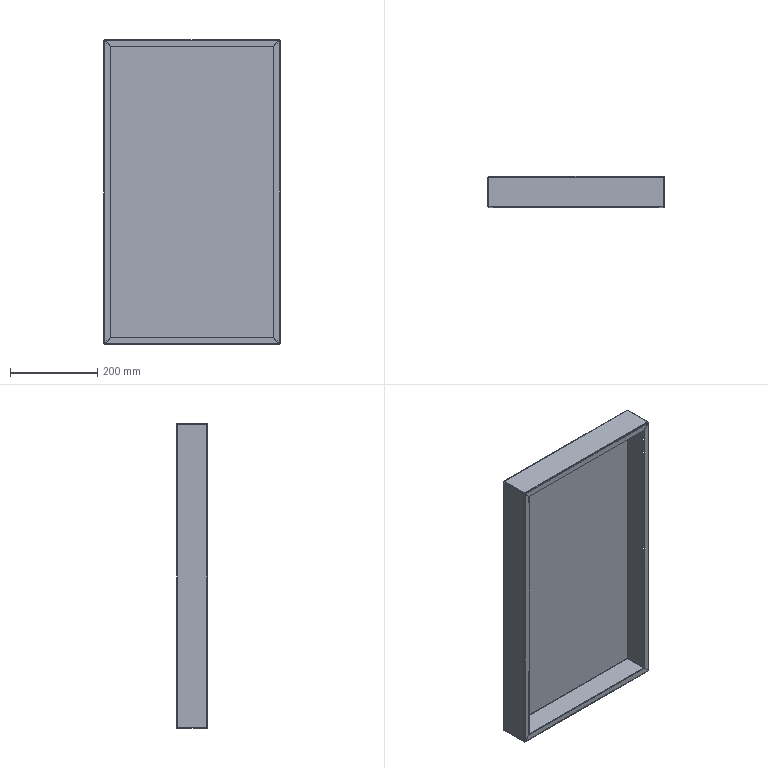Part | SolidWorks | features BaseBody 1 | 1 solid | 78 faces | box 405 x 70 x 700 mm | volume 689241 mm3 | plane 38 | cylinder 24 | spline 16 | commonest cylinder face diameters 1.473 x8 4.473 x8 8.5 x8